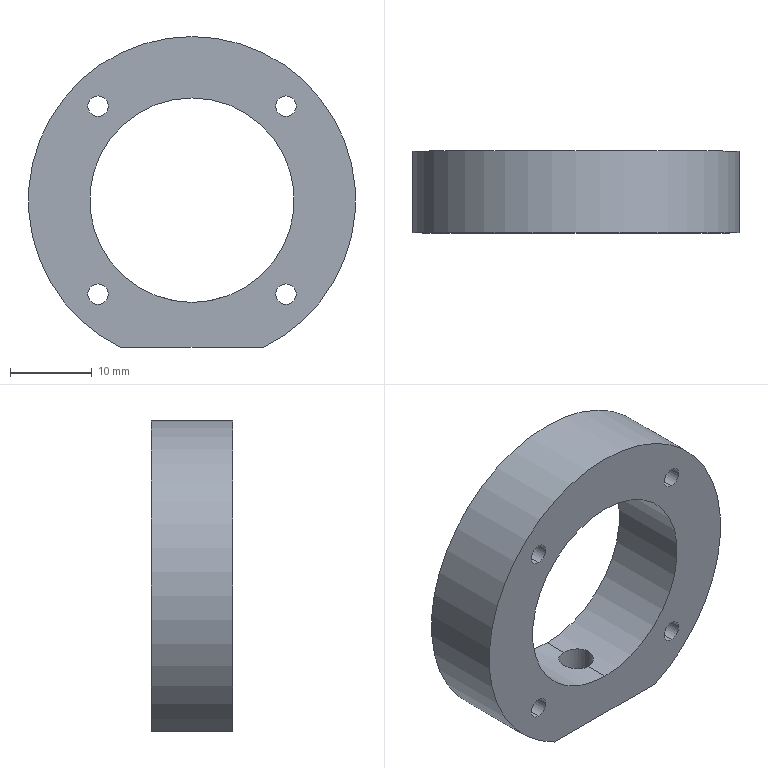Part | SolidWorks | features HoleWzd 2, Extrusion 1, ICE 1 | 1 solid | 16 faces | box 40 x 10 x 38 mm | volume 7150 mm3 | cylinder 13 | plane 3 | commonest cylinder face diameters 2.5 x8 4.2 x2 25 x2 40 x1
STEP:
#1=CARTESIAN_POINT('',(11.49,10.,-12.74));
#2=VERTEX_POINT('',#1);
#3=CARTESIAN_POINT('',(11.49,10.,-10.24));
#4=VERTEX_POINT('',#3);
#5=CARTESIAN_POINT('',(11.49,10.,-11.49));
#6=DIRECTION('',(0.,1.,0.));
#7=DIRECTION('',(0.,0.,1.));
#8=AXIS2_PLACEMENT_3D('',#5,#6,#7);
#9=CIRCLE('',#8,1.25);
#10=EDGE_CURVE('',#2,#4,#9,.T.);
#11=ORIENTED_EDGE('',*,*,#10,.T.);
#12=CARTESIAN_POINT('',(11.49,0.,-10.24));
#13=VERTEX_POINT('',#12);
#14=CARTESIAN_POINT('',(11.49,0.,-10.24));
#15=DIRECTION('',(0.,-1.,0.));
#16=VECTOR('',#15,1000.);
#17=LINE('',#14,#16);
#18=EDGE_CURVE('',#4,#13,#17,.T.);
#19=ORIENTED_EDGE('',*,*,#18,.T.);
#20=CARTESIAN_POINT('',(11.49,0.,-12.74));
#21=VERTEX_POINT('',#20);
#22=CARTESIAN_POINT('',(11.49,0.,-11.49));
#23=DIRECTION('',(0.,-1.,0.));
#24=DIRECTION('',(0.,0.,-1.));
#25=AXIS2_PLACEMENT_3D('',#22,#23,#24);
#26=CIRCLE('',#25,1.25);
#27=EDGE_CURVE('',#13,#21,#26,.T.);
#28=ORIENTED_EDGE('',*,*,#27,.T.);
#29=CARTESIAN_POINT('',(11.49,0.,-12.74));
#30=DIRECTION('',(0.,-1.,0.));
#31=VECTOR('',#30,1000.);
#32=LINE('',#29,#31);
#33=EDGE_CURVE('',#2,#21,#32,.T.);
#34=ORIENTED_EDGE('',*,*,#33,.F.);
#35=EDGE_LOOP('',(#11,#19,#28,#34));
#36=FACE_OUTER_BOUND('',#35,.T.);
#37=CARTESIAN_POINT('',(11.49,0.,-11.49));
#38=DIRECTION('',(0.,-1.,0.));
#39=DIRECTION('',(0.,0.,-1.));
#40=AXIS2_PLACEMENT_3D('',#37,#38,#39);
#41=CYLINDRICAL_SURFACE('',#40,1.25);
#42=ADVANCED_FACE('',(#36),#41,.F.);
#43=CARTESIAN_POINT('',(-11.49,10.,-12.74));
#44=VERTEX_POINT('',#43);
#45=CARTESIAN_POINT('',(-11.49,10.,-10.24));
#46=VERTEX_POINT('',#45);
#47=CARTESIAN_POINT('',(-11.49,10.,-11.49));
#48=DIRECTION('',(0.,1.,0.));
#49=DIRECTION('',(0.,0.,1.));
#50=AXIS2_PLACEMENT_3D('',#47,#48,#49);
#51=CIRCLE('',#50,1.25);
#52=EDGE_CURVE('',#44,#46,#51,.T.);
#53=ORIENTED_EDGE('',*,*,#52,.T.);
#54=CARTESIAN_POINT('',(-11.49,0.,-10.24));
#55=VERTEX_POINT('',#54);
#56=CARTESIAN_POINT('',(-11.49,0.,-10.24));
#57=DIRECTION('',(0.,-1.,0.));
#58=VECTOR('',#57,1000.);
#59=LINE('',#56,#58);
#60=EDGE_CURVE('',#46,#55,#59,.T.);
#61=ORIENTED_EDGE('',*,*,#60,.T.);
#62=CARTESIAN_POINT('',(-11.49,0.,-12.74));
#63=VERTEX_POINT('',#62);
#64=CARTESIAN_POINT('',(-11.49,0.,-11.49));
#65=DIRECTION('',(0.,-1.,0.));
#66=DIRECTION('',(0.,0.,-1.));
#67=AXIS2_PLACEMENT_3D('',#64,#65,#66);
#68=CIRCLE('',#67,1.25);
#69=EDGE_CURVE('',#55,#63,#68,.T.);
#70=ORIENTED_EDGE('',*,*,#69,.T.);
#71=CARTESIAN_POINT('',(-11.49,0.,-12.74));
#72=DIRECTION('',(0.,-1.,0.));
#73=VECTOR('',#72,1000.);
#74=LINE('',#71,#73);
#75=EDGE_CURVE('',#44,#63,#74,.T.);
#76=ORIENTED_EDGE('',*,*,#75,.F.);
#77=EDGE_LOOP('',(#53,#61,#70,#76));
#78=FACE_OUTER_BOUND('',#77,.T.);
#79=CARTESIAN_POINT('',(-11.49,0.,-11.49));
#80=DIRECTION('',(0.,-1.,0.));
#81=DIRECTION('',(0.,0.,-1.));
#82=AXIS2_PLACEMENT_3D('',#79,#80,#81);
#83=CYLINDRICAL_SURFACE('',#82,1.25);
#84=ADVANCED_FACE('',(#78),#83,.F.);
#85=CARTESIAN_POINT('',(11.49,10.,10.24));
#86=VERTEX_POINT('',#85);
#87=CARTESIAN_POINT('',(11.49,10.,12.74));
#88=VERTEX_POINT('',#87);
#89=CARTESIAN_POINT('',(11.49,10.,11.49));
#90=DIRECTION('',(0.,1.,0.));
#91=DIRECTION('',(0.,0.,1.));
#92=AXIS2_PLACEMENT_3D('',#89,#90,#91);
#93=CIRCLE('',#92,1.25);
#94=EDGE_CURVE('',#86,#88,#93,.T.);
#95=ORIENTED_EDGE('',*,*,#94,.T.);
#96=CARTESIAN_POINT('',(11.49,0.,12.74));
#97=VERTEX_POINT('',#96);
#98=CARTESIAN_POINT('',(11.49,0.,12.74));
#99=DIRECTION('',(0.,-1.,0.));
#100=VECTOR('',#99,1000.);
#101=LINE('',#98,#100);
#102=EDGE_CURVE('',#88,#97,#101,.T.);
#103=ORIENTED_EDGE('',*,*,#102,.T.);
#104=CARTESIAN_POINT('',(11.49,0.,10.24));
#105=VERTEX_POINT('',#104);
#106=CARTESIAN_POINT('',(11.49,0.,11.49));
#107=DIRECTION('',(0.,-1.,0.));
#108=DIRECTION('',(0.,0.,-1.));
#109=AXIS2_PLACEMENT_3D('',#106,#107,#108);
#110=CIRCLE('',#109,1.25);
#111=EDGE_CURVE('',#97,#105,#110,.T.);
#112=ORIENTED_EDGE('',*,*,#111,.T.);
#113=CARTESIAN_POINT('',(11.49,0.,10.24));
#114=DIRECTION('',(0.,-1.,0.));
#115=VECTOR('',#114,1000.);
#116=LINE('',#113,#115);
#117=EDGE_CURVE('',#86,#105,#116,.T.);
#118=ORIENTED_EDGE('',*,*,#117,.F.);
#119=EDGE_LOOP('',(#95,#103,#112,#118));
#120=FACE_OUTER_BOUND('',#119,.T.);
#121=CARTESIAN_POINT('',(11.49,0.,11.49));
#122=DIRECTION('',(0.,-1.,0.));
#123=DIRECTION('',(0.,0.,-1.));
#124=AXIS2_PLACEMENT_3D('',#121,#122,#123);
#125=CYLINDRICAL_SURFACE('',#124,1.25);
#126=ADVANCED_FACE('',(#120),#125,.F.);
#127=CARTESIAN_POINT('',(-11.49,10.,10.24));
#128=VERTEX_POINT('',#127);
#129=CARTESIAN_POINT('',(-11.49,10.,12.74));
#130=VERTEX_POINT('',#129);
#131=CARTESIAN_POINT('',(-11.49,10.,11.49));
#132=DIRECTION('',(0.,1.,0.));
#133=DIRECTION('',(0.,0.,1.));
#134=AXIS2_PLACEMENT_3D('',#131,#132,#133);
#135=CIRCLE('',#134,1.25);
#136=EDGE_CURVE('',#128,#130,#135,.T.);
#137=ORIENTED_EDGE('',*,*,#136,.T.);
#138=CARTESIAN_POINT('',(-11.49,0.,12.74));
#139=VERTEX_POINT('',#138);
#140=CARTESIAN_POINT('',(-11.49,0.,12.74));
#141=DIRECTION('',(0.,-1.,0.));
#142=VECTOR('',#141,1000.);
#143=LINE('',#140,#142);
#144=EDGE_CURVE('',#130,#139,#143,.T.);
#145=ORIENTED_EDGE('',*,*,#144,.T.);
#146=CARTESIAN_POINT('',(-11.49,0.,10.24));
#147=VERTEX_POINT('',#146);
#148=CARTESIAN_POINT('',(-11.49,0.,11.49));
#149=DIRECTION('',(0.,-1.,0.));
#150=DIRECTION('',(0.,0.,-1.));
#151=AXIS2_PLACEMENT_3D('',#148,#149,#150);
#152=CIRCLE('',#151,1.25);
#153=EDGE_CURVE('',#139,#147,#152,.T.);
#154=ORIENTED_EDGE('',*,*,#153,.T.);
#155=CARTESIAN_POINT('',(-11.49,0.,10.24));
#156=DIRECTION('',(0.,-1.,0.));
#157=VECTOR('',#156,1000.);
#158=LINE('',#155,#157);
#159=EDGE_CURVE('',#128,#147,#158,.T.);
#160=ORIENTED_EDGE('',*,*,#159,.F.);
#161=EDGE_LOOP('',(#137,#145,#154,#160));
#162=FACE_OUTER_BOUND('',#161,.T.);
#163=CARTESIAN_POINT('',(-11.49,0.,11.49));
#164=DIRECTION('',(0.,-1.,0.));
#165=DIRECTION('',(0.,0.,-1.));
#166=AXIS2_PLACEMENT_3D('',#163,#164,#165);
#167=CYLINDRICAL_SURFACE('',#166,1.25);
#168=ADVANCED_FACE('',(#162),#167,.F.);
#169=CARTESIAN_POINT('',(0.,2.9,-12.5));
#170=VERTEX_POINT('',#169);
#171=CARTESIAN_POINT('',(2.1,5.,-12.322));
#172=VERTEX_POINT('',#171);
#173=CARTESIAN_POINT('',(0.,2.9,-12.5));
#174=CARTESIAN_POINT('',(0.2744,2.9,-12.5));
#175=CARTESIAN_POINT('',(0.5513,2.955,-12.49));
#176=CARTESIAN_POINT('',(0.9305,3.112,-12.466));
#177=CARTESIAN_POINT('',(1.053,3.178,-12.456));
#178=CARTESIAN_POINT('',(1.282,3.331,-12.435));
#179=CARTESIAN_POINT('',(1.388,3.418,-12.423));
#180=CARTESIAN_POINT('',(1.581,3.611,-12.4));
#181=CARTESIAN_POINT('',(1.67,3.719,-12.388));
#182=CARTESIAN_POINT('',(1.822,3.947,-12.367));
#183=CARTESIAN_POINT('',(1.887,4.068,-12.357));
#184=CARTESIAN_POINT('',(1.992,4.322,-12.34));
#185=CARTESIAN_POINT('',(2.033,4.455,-12.334));
#186=CARTESIAN_POINT('',(2.086,4.724,-12.325));
#187=CARTESIAN_POINT('',(2.1,4.861,-12.322));
#188=CARTESIAN_POINT('',(2.1,5.,-12.322));
#189=B_SPLINE_CURVE_WITH_KNOTS('',3,(#173,#174,#175,#176,#177,#178,#179,#180,#181,#182,#183,#184,#185,#186,#187,#188),.UNSPECIFIED.,.F.,.F.,(4,2,2,2,2,2,2,4),(0.006577,0.007399,0.007811,0.008222,0.008633,0.009044,0.009455,0.009866),.UNSPECIFIED.);
#190=EDGE_CURVE('',#170,#172,#189,.T.);
#191=ORIENTED_EDGE('',*,*,#190,.T.);
#192=CARTESIAN_POINT('',(2.1,5.,-18.));
#193=VERTEX_POINT('',#192);
#194=CARTESIAN_POINT('',(2.1,5.,-18.));
#195=DIRECTION('',(0.,0.,-1.));
#196=VECTOR('',#195,1000.);
#197=LINE('',#194,#196);
#198=EDGE_CURVE('',#172,#193,#197,.T.);
#199=ORIENTED_EDGE('',*,*,#198,.T.);
#200=CARTESIAN_POINT('',(-2.1,5.,-18.));
#201=VERTEX_POINT('',#200);
#202=CARTESIAN_POINT('',(0.,5.,-18.));
#203=DIRECTION('',(0.,0.,-1.));
#204=DIRECTION('',(-1.,0.,0.));
#205=AXIS2_PLACEMENT_3D('',#202,#203,#204);
#206=CIRCLE('',#205,2.1);
#207=EDGE_CURVE('',#193,#201,#206,.T.);
#208=ORIENTED_EDGE('',*,*,#207,.T.);
#209=CARTESIAN_POINT('',(-2.1,5.,-12.322));
#210=VERTEX_POINT('',#209);
#211=CARTESIAN_POINT('',(-2.1,5.,-18.));
#212=DIRECTION('',(0.,0.,-1.));
#213=VECTOR('',#212,1000.);
#214=LINE('',#211,#213);
#215=EDGE_CURVE('',#210,#201,#214,.T.);
#216=ORIENTED_EDGE('',*,*,#215,.F.);
#217=CARTESIAN_POINT('',(-2.1,5.,-12.322));
#218=CARTESIAN_POINT('',(-2.1,4.863,-12.322));
#219=CARTESIAN_POINT('',(-2.086,4.723,-12.325));
#220=CARTESIAN_POINT('',(-2.032,4.454,-12.334));
#221=CARTESIAN_POINT('',(-1.993,4.323,-12.34));
#222=CARTESIAN_POINT('',(-1.887,4.068,-12.357));
#223=CARTESIAN_POINT('',(-1.821,3.946,-12.367));
#224=CARTESIAN_POINT('',(-1.669,3.719,-12.388));
#225=CARTESIAN_POINT('',(-1.582,3.613,-12.4));
#226=CARTESIAN_POINT('',(-1.387,3.417,-12.423));
#227=CARTESIAN_POINT('',(-1.281,3.33,-12.435));
#228=CARTESIAN_POINT('',(-1.054,3.178,-12.456));
#229=CARTESIAN_POINT('',(-0.931,3.113,-12.466));
#230=CARTESIAN_POINT('',(-0.677,3.007,-12.482));
#231=CARTESIAN_POINT('',(-0.5461,2.968,-12.489));
#232=CARTESIAN_POINT('',(-0.2765,2.914,-12.498));
#233=CARTESIAN_POINT('',(-0.1372,2.9,-12.5));
#234=CARTESIAN_POINT('',(0.,2.9,-12.5));
#235=B_SPLINE_CURVE_WITH_KNOTS('',3,(#217,#218,#219,#220,#221,#222,#223,#224,#225,#226,#227,#228,#229,#230,#231,#232,#233,#234),.UNSPECIFIED.,.F.,.F.,(4,2,2,2,2,2,2,2,4),(0.003289,0.0037,0.004111,0.004522,0.004933,0.005344,0.005755,0.006166,0.006577),.UNSPECIFIED.);
#236=EDGE_CURVE('',#210,#170,#235,.T.);
#237=ORIENTED_EDGE('',*,*,#236,.T.);
#238=EDGE_LOOP('',(#191,#199,#208,#216,#237));
#239=FACE_OUTER_BOUND('',#238,.T.);
#240=CARTESIAN_POINT('',(0.,5.,-18.));
#241=DIRECTION('',(0.,0.,-1.));
#242=DIRECTION('',(-1.,0.,0.));
#243=AXIS2_PLACEMENT_3D('',#240,#241,#242);
#244=CYLINDRICAL_SURFACE('',#243,2.1);
#245=ADVANCED_FACE('',(#239),#244,.F.);
#246=CARTESIAN_POINT('',(0.,10.,-12.5));
#247=VERTEX_POINT('',#246);
#248=CARTESIAN_POINT('',(0.,10.,12.5));
#249=VERTEX_POINT('',#248);
#250=CARTESIAN_POINT('',(0.,10.,0.));
#251=DIRECTION('',(0.,1.,0.));
#252=DIRECTION('',(0.,0.,1.));
#253=AXIS2_PLACEMENT_3D('',#250,#251,#252);
#254=CIRCLE('',#253,12.5);
#255=EDGE_CURVE('',#247,#249,#254,.T.);
#256=ORIENTED_EDGE('',*,*,#255,.T.);
#257=CARTESIAN_POINT('',(0.,0.,12.5));
#258=VERTEX_POINT('',#257);
#259=CARTESIAN_POINT('',(0.,10.,12.5));
#260=DIRECTION('',(0.,-1.,0.));
#261=VECTOR('',#260,1000.);
#262=LINE('',#259,#261);
#263=EDGE_CURVE('',#249,#258,#262,.T.);
#264=ORIENTED_EDGE('',*,*,#263,.T.);
#265=CARTESIAN_POINT('',(0.,0.,-12.5));
#266=VERTEX_POINT('',#265);
#267=CARTESIAN_POINT('',(0.,0.,0.));
#268=DIRECTION('',(0.,1.,0.));
#269=DIRECTION('',(0.,0.,1.));
#270=AXIS2_PLACEMENT_3D('',#267,#268,#269);
#271=CIRCLE('',#270,12.5);
#272=EDGE_CURVE('',#266,#258,#271,.T.);
#273=ORIENTED_EDGE('',*,*,#272,.F.);
#274=CARTESIAN_POINT('',(0.,10.,-12.5));
#275=DIRECTION('',(0.,-1.,0.));
#276=VECTOR('',#275,1000.);
#277=LINE('',#274,#276);
#278=EDGE_CURVE('',#170,#266,#277,.T.);
#279=ORIENTED_EDGE('',*,*,#278,.F.);
#280=ORIENTED_EDGE('',*,*,#236,.F.);
#281=CARTESIAN_POINT('',(0.,7.1,-12.5));
#282=VERTEX_POINT('',#281);
#283=CARTESIAN_POINT('',(0.,7.1,-12.5));
#284=CARTESIAN_POINT('',(-0.1391,7.1,-12.5));
#285=CARTESIAN_POINT('',(-0.2757,7.086,-12.498));
#286=CARTESIAN_POINT('',(-0.5445,7.033,-12.489));
#287=CARTESIAN_POINT('',(-0.6781,6.992,-12.482));
#288=CARTESIAN_POINT('',(-0.9324,6.887,-12.466));
#289=CARTESIAN_POINT('',(-1.053,6.822,-12.456));
#290=CARTESIAN_POINT('',(-1.281,6.67,-12.435));
#291=CARTESIAN_POINT('',(-1.389,6.581,-12.423));
#292=CARTESIAN_POINT('',(-1.679,6.291,-12.388));
#293=CARTESIAN_POINT('',(-1.835,6.057,-12.365));
#294=CARTESIAN_POINT('',(-2.045,5.551,-12.332));
#295=CARTESIAN_POINT('',(-2.1,5.275,-12.322));
#296=CARTESIAN_POINT('',(-2.1,5.,-12.322));
#297=B_SPLINE_CURVE_WITH_KNOTS('',3,(#283,#284,#285,#286,#287,#288,#289,#290,#291,#292,#293,#294,#295,#296),.UNSPECIFIED.,.F.,.F.,(4,2,2,2,2,2,4),(0.,0.0004112,0.0008224,0.001234,0.001645,0.002467,0.003289),.UNSPECIFIED.);
#298=EDGE_CURVE('',#282,#210,#297,.T.);
#299=ORIENTED_EDGE('',*,*,#298,.F.);
#300=CARTESIAN_POINT('',(0.,10.,-12.5));
#301=DIRECTION('',(0.,-1.,0.));
#302=VECTOR('',#301,1000.);
#303=LINE('',#300,#302);
#304=EDGE_CURVE('',#247,#282,#303,.T.);
#305=ORIENTED_EDGE('',*,*,#304,.F.);
#306=EDGE_LOOP('',(#256,#264,#273,#279,#280,#299,#305));
#307=FACE_OUTER_BOUND('',#306,.T.);
#308=CARTESIAN_POINT('',(0.,10.,0.));
#309=DIRECTION('',(0.,-1.,0.));
#310=DIRECTION('',(0.,0.,-1.));
#311=AXIS2_PLACEMENT_3D('',#308,#309,#310);
#312=CYLINDRICAL_SURFACE('',#311,12.5);
#313=ADVANCED_FACE('',(#307),#312,.F.);
#314=CARTESIAN_POINT('',(11.49,0.,11.49));
#315=DIRECTION('',(0.,-1.,0.));
#316=DIRECTION('',(0.,0.,-1.));
#317=AXIS2_PLACEMENT_3D('',#314,#315,#316);
#318=CIRCLE('',#317,1.25);
#319=EDGE_CURVE('',#105,#97,#318,.T.);
#320=ORIENTED_EDGE('',*,*,#319,.F.);
#321=ORIENTED_EDGE('',*,*,#111,.F.);
#322=EDGE_LOOP('',(#320,#321));
#323=FACE_BOUND('',#322,.T.);
#324=CARTESIAN_POINT('',(-8.718,0.,-18.));
#325=VERTEX_POINT('',#324);
#326=CARTESIAN_POINT('',(8.718,0.,-18.));
#327=VERTEX_POINT('',#326);
#328=CARTESIAN_POINT('',(0.,0.,0.));
#329=DIRECTION('',(0.,1.,0.));
#330=DIRECTION('',(0.,0.,1.));
#331=AXIS2_PLACEMENT_3D('',#328,#329,#330);
#332=CIRCLE('',#331,20.);
#333=EDGE_CURVE('',#325,#327,#332,.T.);
#334=ORIENTED_EDGE('',*,*,#333,.F.);
#335=CARTESIAN_POINT('',(8.718,0.,-18.));
#336=DIRECTION('',(1.,0.,0.));
#337=VECTOR('',#336,1000.);
#338=LINE('',#335,#337);
#339=EDGE_CURVE('',#325,#327,#338,.T.);
#340=ORIENTED_EDGE('',*,*,#339,.T.);
#341=EDGE_LOOP('',(#334,#340));
#342=FACE_OUTER_BOUND('',#341,.T.);
#343=ORIENTED_EDGE('',*,*,#272,.T.);
#344=CARTESIAN_POINT('',(0.,0.,0.));
#345=DIRECTION('',(0.,1.,0.));
#346=DIRECTION('',(0.,0.,1.));
#347=AXIS2_PLACEMENT_3D('',#344,#345,#346);
#348=CIRCLE('',#347,12.5);
#349=EDGE_CURVE('',#258,#266,#348,.T.);
#350=ORIENTED_EDGE('',*,*,#349,.T.);
#351=EDGE_LOOP('',(#343,#350));
#352=FACE_BOUND('',#351,.T.);
#353=CARTESIAN_POINT('',(-11.49,0.,11.49));
#354=DIRECTION('',(0.,-1.,0.));
#355=DIRECTION('',(0.,0.,-1.));
#356=AXIS2_PLACEMENT_3D('',#353,#354,#355);
#357=CIRCLE('',#356,1.25);
#358=EDGE_CURVE('',#147,#139,#357,.T.);
#359=ORIENTED_EDGE('',*,*,#358,.F.);
#360=ORIENTED_EDGE('',*,*,#153,.F.);
#361=EDGE_LOOP('',(#359,#360));
#362=FACE_BOUND('',#361,.T.);
#363=CARTESIAN_POINT('',(-11.49,0.,-11.49));
#364=DIRECTION('',(0.,-1.,0.));
#365=DIRECTION('',(0.,0.,-1.));
#366=AXIS2_PLACEMENT_3D('',#363,#364,#365);
#367=CIRCLE('',#366,1.25);
#368=EDGE_CURVE('',#63,#55,#367,.T.);
#369=ORIENTED_EDGE('',*,*,#368,.F.);
#370=ORIENTED_EDGE('',*,*,#69,.F.);
#371=EDGE_LOOP('',(#369,#370));
#372=FACE_BOUND('',#371,.T.);
#373=CARTESIAN_POINT('',(11.49,0.,-11.49));
#374=DIRECTION('',(0.,-1.,0.));
#375=DIRECTION('',(0.,0.,-1.));
#376=AXIS2_PLACEMENT_3D('',#373,#374,#375);
#377=CIRCLE('',#376,1.25);
#378=EDGE_CURVE('',#21,#13,#377,.T.);
#379=ORIENTED_EDGE('',*,*,#378,.F.);
#380=ORIENTED_EDGE('',*,*,#27,.F.);
#381=EDGE_LOOP('',(#379,#380));
#382=FACE_BOUND('',#381,.T.);
#383=CARTESIAN_POINT('',(0.,0.,0.));
#384=DIRECTION('',(0.,1.,0.));
#385=DIRECTION('',(0.,0.,1.));
#386=AXIS2_PLACEMENT_3D('',#383,#384,#385);
#387=PLANE('',#386);
#388=ADVANCED_FACE('',(#323,#342,#352,#362,#372,#382),#387,.F.);
#389=ORIENTED_EDGE('',*,*,#10,.F.);
#390=CARTESIAN_POINT('',(11.49,10.,-11.49));
#391=DIRECTION('',(0.,1.,0.));
#392=DIRECTION('',(0.,0.,1.));
#393=AXIS2_PLACEMENT_3D('',#390,#391,#392);
#394=CIRCLE('',#393,1.25);
#395=EDGE_CURVE('',#4,#2,#394,.T.);
#396=ORIENTED_EDGE('',*,*,#395,.F.);
#397=EDGE_LOOP('',(#389,#396));
#398=FACE_BOUND('',#397,.T.);
#399=ORIENTED_EDGE('',*,*,#52,.F.);
#400=CARTESIAN_POINT('',(-11.49,10.,-11.49));
#401=DIRECTION('',(0.,1.,0.));
#402=DIRECTION('',(0.,0.,1.));
#403=AXIS2_PLACEMENT_3D('',#400,#401,#402);
#404=CIRCLE('',#403,1.25);
#405=EDGE_CURVE('',#46,#44,#404,.T.);
#406=ORIENTED_EDGE('',*,*,#405,.F.);
#407=EDGE_LOOP('',(#399,#406));
#408=FACE_BOUND('',#407,.T.);
#409=ORIENTED_EDGE('',*,*,#94,.F.);
#410=CARTESIAN_POINT('',(11.49,10.,11.49));
#411=DIRECTION('',(0.,1.,0.));
#412=DIRECTION('',(0.,0.,1.));
#413=AXIS2_PLACEMENT_3D('',#410,#411,#412);
#414=CIRCLE('',#413,1.25);
#415=EDGE_CURVE('',#88,#86,#414,.T.);
#416=ORIENTED_EDGE('',*,*,#415,.F.);
#417=EDGE_LOOP('',(#409,#416));
#418=FACE_BOUND('',#417,.T.);
#419=ORIENTED_EDGE('',*,*,#136,.F.);
#420=CARTESIAN_POINT('',(-11.49,10.,11.49));
#421=DIRECTION('',(0.,1.,0.));
#422=DIRECTION('',(0.,0.,1.));
#423=AXIS2_PLACEMENT_3D('',#420,#421,#422);
#424=CIRCLE('',#423,1.25);
#425=EDGE_CURVE('',#130,#128,#424,.T.);
#426=ORIENTED_EDGE('',*,*,#425,.F.);
#427=EDGE_LOOP('',(#419,#426));
#428=FACE_BOUND('',#427,.T.);
#429=CARTESIAN_POINT('',(-8.718,10.,-18.));
#430=VERTEX_POINT('',#429);
#431=CARTESIAN_POINT('',(8.718,10.,-18.));
#432=VERTEX_POINT('',#431);
#433=CARTESIAN_POINT('',(8.718,10.,-18.));
#434=DIRECTION('',(1.,0.,0.));
#435=VECTOR('',#434,1000.);
#436=LINE('',#433,#435);
#437=EDGE_CURVE('',#430,#432,#436,.T.);
#438=ORIENTED_EDGE('',*,*,#437,.F.);
#439=CARTESIAN_POINT('',(0.,10.,0.));
#440=DIRECTION('',(0.,1.,0.));
#441=DIRECTION('',(0.,0.,1.));
#442=AXIS2_PLACEMENT_3D('',#439,#440,#441);
#443=CIRCLE('',#442,20.);
#444=EDGE_CURVE('',#430,#432,#443,.T.);
#445=ORIENTED_EDGE('',*,*,#444,.T.);
#446=EDGE_LOOP('',(#438,#445));
#447=FACE_OUTER_BOUND('',#446,.T.);
#448=ORIENTED_EDGE('',*,*,#255,.F.);
#449=CARTESIAN_POINT('',(0.,10.,0.));
#450=DIRECTION('',(0.,1.,0.));
#451=DIRECTION('',(0.,0.,1.));
#452=AXIS2_PLACEMENT_3D('',#449,#450,#451);
#453=CIRCLE('',#452,12.5);
#454=EDGE_CURVE('',#249,#247,#453,.T.);
#455=ORIENTED_EDGE('',*,*,#454,.F.);
#456=EDGE_LOOP('',(#448,#455));
#457=FACE_BOUND('',#456,.T.);
#458=CARTESIAN_POINT('',(0.,10.,0.));
#459=DIRECTION('',(0.,1.,0.));
#460=DIRECTION('',(0.,0.,1.));
#461=AXIS2_PLACEMENT_3D('',#458,#459,#460);
#462=PLANE('',#461);
#463=ADVANCED_FACE('',(#398,#408,#418,#428,#447,#457),#462,.T.);
#464=ORIENTED_EDGE('',*,*,#444,.F.);
#465=CARTESIAN_POINT('',(-8.718,0.,-18.));
#466=DIRECTION('',(0.,1.,0.));
#467=VECTOR('',#466,1000.);
#468=LINE('',#465,#467);
#469=EDGE_CURVE('',#325,#430,#468,.T.);
#470=ORIENTED_EDGE('',*,*,#469,.F.);
#471=ORIENTED_EDGE('',*,*,#333,.T.);
#472=CARTESIAN_POINT('',(8.718,0.,-18.));
#473=DIRECTION('',(0.,1.,0.));
#474=VECTOR('',#473,1000.);
#475=LINE('',#472,#474);
#476=EDGE_CURVE('',#327,#432,#475,.T.);
#477=ORIENTED_EDGE('',*,*,#476,.T.);
#478=EDGE_LOOP('',(#464,#470,#471,#477));
#479=FACE_OUTER_BOUND('',#478,.T.);
#480=CARTESIAN_POINT('',(0.,10.,0.));
#481=DIRECTION('',(0.,-1.,0.));
#482=DIRECTION('',(0.,0.,-1.));
#483=AXIS2_PLACEMENT_3D('',#480,#481,#482);
#484=CYLINDRICAL_SURFACE('',#483,20.);
#485=ADVANCED_FACE('',(#479),#484,.T.);
#486=ORIENTED_EDGE('',*,*,#263,.F.);
#487=ORIENTED_EDGE('',*,*,#454,.T.);
#488=ORIENTED_EDGE('',*,*,#304,.T.);
#489=CARTESIAN_POINT('',(2.1,5.,-12.322));
#490=CARTESIAN_POINT('',(2.1,5.139,-12.322));
#491=CARTESIAN_POINT('',(2.086,5.275,-12.325));
#492=CARTESIAN_POINT('',(2.033,5.544,-12.334));
#493=CARTESIAN_POINT('',(1.992,5.678,-12.34));
#494=CARTESIAN_POINT('',(1.887,5.931,-12.357));
#495=CARTESIAN_POINT('',(1.823,6.052,-12.367));
#496=CARTESIAN_POINT('',(1.67,6.28,-12.388));
#497=CARTESIAN_POINT('',(1.582,6.388,-12.4));
#498=CARTESIAN_POINT('',(1.292,6.678,-12.435));
#499=CARTESIAN_POINT('',(1.059,6.834,-12.458));
#500=CARTESIAN_POINT('',(0.6801,6.992,-12.482));
#501=CARTESIAN_POINT('',(0.5473,7.032,-12.489));
#502=CARTESIAN_POINT('',(0.2762,7.086,-12.498));
#503=CARTESIAN_POINT('',(0.1389,7.1,-12.5));
#504=CARTESIAN_POINT('',(0.,7.1,-12.5));
#505=B_SPLINE_CURVE_WITH_KNOTS('',3,(#489,#490,#491,#492,#493,#494,#495,#496,#497,#498,#499,#500,#501,#502,#503,#504),.UNSPECIFIED.,.F.,.F.,(4,2,2,2,2,2,2,4),(0.009866,0.01028,0.01069,0.0111,0.01151,0.01233,0.01274,0.01315),.UNSPECIFIED.);
#506=EDGE_CURVE('',#172,#282,#505,.T.);
#507=ORIENTED_EDGE('',*,*,#506,.F.);
#508=ORIENTED_EDGE('',*,*,#190,.F.);
#509=ORIENTED_EDGE('',*,*,#278,.T.);
#510=ORIENTED_EDGE('',*,*,#349,.F.);
#511=EDGE_LOOP('',(#486,#487,#488,#507,#508,#509,#510));
#512=FACE_OUTER_BOUND('',#511,.T.);
#513=CARTESIAN_POINT('',(0.,10.,0.));
#514=DIRECTION('',(0.,-1.,0.));
#515=DIRECTION('',(0.,0.,-1.));
#516=AXIS2_PLACEMENT_3D('',#513,#514,#515);
#517=CYLINDRICAL_SURFACE('',#516,12.5);
#518=ADVANCED_FACE('',(#512),#517,.F.);
#519=CARTESIAN_POINT('',(0.,5.,-18.));
#520=DIRECTION('',(0.,0.,-1.));
#521=DIRECTION('',(-1.,0.,0.));
#522=AXIS2_PLACEMENT_3D('',#519,#520,#521);
#523=CIRCLE('',#522,2.1);
#524=EDGE_CURVE('',#201,#193,#523,.T.);
#525=ORIENTED_EDGE('',*,*,#524,.F.);
#526=ORIENTED_EDGE('',*,*,#207,.F.);
#527=EDGE_LOOP('',(#525,#526));
#528=FACE_BOUND('',#527,.T.);
#529=ORIENTED_EDGE('',*,*,#437,.T.);
#530=ORIENTED_EDGE('',*,*,#476,.F.);
#531=ORIENTED_EDGE('',*,*,#339,.F.);
#532=ORIENTED_EDGE('',*,*,#469,.T.);
#533=EDGE_LOOP('',(#529,#530,#531,#532));
#534=FACE_OUTER_BOUND('',#533,.T.);
#535=CARTESIAN_POINT('',(8.718,0.,-18.));
#536=DIRECTION('',(0.,0.,1.));
#537=DIRECTION('',(1.,0.,0.));
#538=AXIS2_PLACEMENT_3D('',#535,#536,#537);
#539=PLANE('',#538);
#540=ADVANCED_FACE('',(#528,#534),#539,.F.);
#541=ORIENTED_EDGE('',*,*,#198,.F.);
#542=ORIENTED_EDGE('',*,*,#506,.T.);
#543=ORIENTED_EDGE('',*,*,#298,.T.);
#544=ORIENTED_EDGE('',*,*,#215,.T.);
#545=ORIENTED_EDGE('',*,*,#524,.T.);
#546=EDGE_LOOP('',(#541,#542,#543,#544,#545));
#547=FACE_OUTER_BOUND('',#546,.T.);
#548=CARTESIAN_POINT('',(0.,5.,-18.));
#549=DIRECTION('',(0.,0.,-1.));
#550=DIRECTION('',(-1.,0.,0.));
#551=AXIS2_PLACEMENT_3D('',#548,#549,#550);
#552=CYLINDRICAL_SURFACE('',#551,2.1);
#553=ADVANCED_FACE('',(#547),#552,.F.);
#554=ORIENTED_EDGE('',*,*,#144,.F.);
#555=ORIENTED_EDGE('',*,*,#425,.T.);
#556=ORIENTED_EDGE('',*,*,#159,.T.);
#557=ORIENTED_EDGE('',*,*,#358,.T.);
#558=EDGE_LOOP('',(#554,#555,#556,#557));
#559=FACE_OUTER_BOUND('',#558,.T.);
#560=CARTESIAN_POINT('',(-11.49,0.,11.49));
#561=DIRECTION('',(0.,-1.,0.));
#562=DIRECTION('',(0.,0.,-1.));
#563=AXIS2_PLACEMENT_3D('',#560,#561,#562);
#564=CYLINDRICAL_SURFACE('',#563,1.25);
#565=ADVANCED_FACE('',(#559),#564,.F.);
#566=ORIENTED_EDGE('',*,*,#102,.F.);
#567=ORIENTED_EDGE('',*,*,#415,.T.);
#568=ORIENTED_EDGE('',*,*,#117,.T.);
#569=ORIENTED_EDGE('',*,*,#319,.T.);
#570=EDGE_LOOP('',(#566,#567,#568,#569));
#571=FACE_OUTER_BOUND('',#570,.T.);
#572=CARTESIAN_POINT('',(11.49,0.,11.49));
#573=DIRECTION('',(0.,-1.,0.));
#574=DIRECTION('',(0.,0.,-1.));
#575=AXIS2_PLACEMENT_3D('',#572,#573,#574);
#576=CYLINDRICAL_SURFACE('',#575,1.25);
#577=ADVANCED_FACE('',(#571),#576,.F.);
#578=ORIENTED_EDGE('',*,*,#60,.F.);
#579=ORIENTED_EDGE('',*,*,#405,.T.);
#580=ORIENTED_EDGE('',*,*,#75,.T.);
#581=ORIENTED_EDGE('',*,*,#368,.T.);
#582=EDGE_LOOP('',(#578,#579,#580,#581));
#583=FACE_OUTER_BOUND('',#582,.T.);
#584=CARTESIAN_POINT('',(-11.49,0.,-11.49));
#585=DIRECTION('',(0.,-1.,0.));
#586=DIRECTION('',(0.,0.,-1.));
#587=AXIS2_PLACEMENT_3D('',#584,#585,#586);
#588=CYLINDRICAL_SURFACE('',#587,1.25);
#589=ADVANCED_FACE('',(#583),#588,.F.);
#590=ORIENTED_EDGE('',*,*,#18,.F.);
#591=ORIENTED_EDGE('',*,*,#395,.T.);
#592=ORIENTED_EDGE('',*,*,#33,.T.);
#593=ORIENTED_EDGE('',*,*,#378,.T.);
#594=EDGE_LOOP('',(#590,#591,#592,#593));
#595=FACE_OUTER_BOUND('',#594,.T.);
#596=CARTESIAN_POINT('',(11.49,0.,-11.49));
#597=DIRECTION('',(0.,-1.,0.));
#598=DIRECTION('',(0.,0.,-1.));
#599=AXIS2_PLACEMENT_3D('',#596,#597,#598);
#600=CYLINDRICAL_SURFACE('',#599,1.25);
#601=ADVANCED_FACE('',(#595),#600,.F.);
#602=CLOSED_SHELL('',(#42,#84,#126,#168,#245,#313,#388,#463,#485,#518,#540,#553,#565,#577,#589,#601));
#603=MANIFOLD_SOLID_BREP('',#602);
#604=CARTESIAN_POINT('',(0.,0.,0.));
#605=DIRECTION('',(0.,0.,1.));
#606=DIRECTION('',(1.,0.,0.));
#607=AXIS2_PLACEMENT_3D('',#604,#605,#606);
#608=(LENGTH_UNIT()NAMED_UNIT(*)SI_UNIT(.MILLI.,.METRE.));
#609=UNCERTAINTY_MEASURE_WITH_UNIT(LENGTH_MEASURE(0.00001),#608,'','');
#610=(NAMED_UNIT(*)PLANE_ANGLE_UNIT()SI_UNIT($,.RADIAN.));
#611=(NAMED_UNIT(*)SI_UNIT($,.STERADIAN.)SOLID_ANGLE_UNIT());
#612=(GEOMETRIC_REPRESENTATION_CONTEXT(3)GLOBAL_UNCERTAINTY_ASSIGNED_CONTEXT((#609))GLOBAL_UNIT_ASSIGNED_CONTEXT((#608,#610,#611))REPRESENTATION_CONTEXT('',''));
#613=ADVANCED_BREP_SHAPE_REPRESENTATION('',(#603,#607),#612);